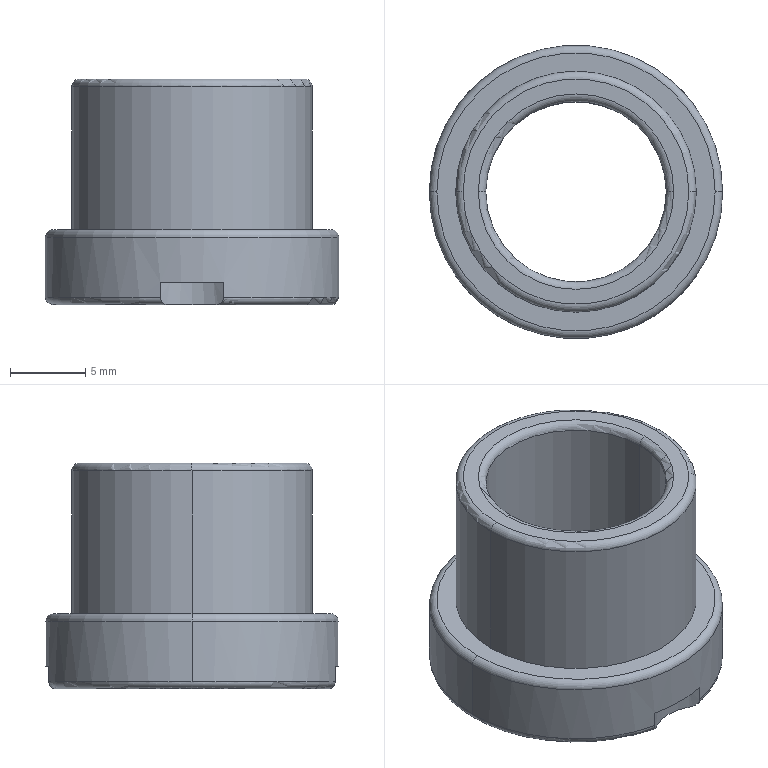Part | SolidWorks | features BaseBody 1 | 1 solid | 24 faces | box 19.5 x 19.5 x 15 mm | volume 1786 mm3 | torus 11 | cylinder 8 | plane 5 | commonest cylinder face diameters 6.5 x2 12 x2 16 x2 19.5 x2
STEP:
#1=CARTESIAN_POINT('',(-8.,0.,14.5));
#2=VERTEX_POINT('',#1);
#3=CARTESIAN_POINT('',(8.,0.,14.5));
#4=VERTEX_POINT('',#3);
#5=CARTESIAN_POINT('',(0.,0.,14.5));
#6=DIRECTION('',(0.,0.,-1.));
#7=DIRECTION('',(1.,0.,0.));
#8=AXIS2_PLACEMENT_3D('',#5,#6,#7);
#9=CIRCLE('',#8,8.);
#10=EDGE_CURVE('',#2,#4,#9,.T.);
#11=ORIENTED_EDGE('',*,*,#10,.F.);
#12=CARTESIAN_POINT('',(-7.5,0.,15.));
#13=VERTEX_POINT('',#12);
#14=CARTESIAN_POINT('',(-7.5,0.,14.5));
#15=DIRECTION('',(0.,1.,0.));
#16=DIRECTION('',(-1.,0.,0.));
#17=AXIS2_PLACEMENT_3D('',#14,#15,#16);
#18=CIRCLE('',#17,0.5);
#19=EDGE_CURVE('',#2,#13,#18,.T.);
#20=ORIENTED_EDGE('',*,*,#19,.T.);
#21=CARTESIAN_POINT('',(7.5,0.,15.));
#22=VERTEX_POINT('',#21);
#23=CARTESIAN_POINT('',(0.,0.,15.));
#24=DIRECTION('',(0.,0.,1.));
#25=DIRECTION('',(1.,0.,0.));
#26=AXIS2_PLACEMENT_3D('',#23,#24,#25);
#27=CIRCLE('',#26,7.5);
#28=EDGE_CURVE('',#22,#13,#27,.T.);
#29=ORIENTED_EDGE('',*,*,#28,.F.);
#30=CARTESIAN_POINT('',(7.5,0.,14.5));
#31=DIRECTION('',(0.,-1.,0.));
#32=DIRECTION('',(0.,0.,-1.));
#33=AXIS2_PLACEMENT_3D('',#30,#31,#32);
#34=CIRCLE('',#33,0.5);
#35=EDGE_CURVE('',#4,#22,#34,.T.);
#36=ORIENTED_EDGE('',*,*,#35,.F.);
#37=EDGE_LOOP('',(#11,#20,#29,#36));
#38=FACE_OUTER_BOUND('',#37,.T.);
#39=CARTESIAN_POINT('',(0.,0.,14.5));
#40=DIRECTION('',(0.,0.,1.));
#41=DIRECTION('',(1.,0.,0.));
#42=AXIS2_PLACEMENT_3D('',#39,#40,#41);
#43=TOROIDAL_SURFACE('',#42,7.5,0.5);
#44=ADVANCED_FACE('',(#38),#43,.T.);
#45=CARTESIAN_POINT('',(9.25,0.,5.));
#46=VERTEX_POINT('',#45);
#47=CARTESIAN_POINT('',(-9.25,0.,5.));
#48=VERTEX_POINT('',#47);
#49=CARTESIAN_POINT('',(0.,0.,5.));
#50=DIRECTION('',(0.,0.,1.));
#51=DIRECTION('',(-1.,0.,0.));
#52=AXIS2_PLACEMENT_3D('',#49,#50,#51);
#53=CIRCLE('',#52,9.25);
#54=EDGE_CURVE('',#46,#48,#53,.T.);
#55=ORIENTED_EDGE('',*,*,#54,.F.);
#56=CARTESIAN_POINT('',(9.75,0.,4.5));
#57=VERTEX_POINT('',#56);
#58=CARTESIAN_POINT('',(9.25,0.,4.5));
#59=DIRECTION('',(0.,1.,0.));
#60=DIRECTION('',(-1.,0.,0.));
#61=AXIS2_PLACEMENT_3D('',#58,#59,#60);
#62=CIRCLE('',#61,0.5);
#63=EDGE_CURVE('',#46,#57,#62,.T.);
#64=ORIENTED_EDGE('',*,*,#63,.T.);
#65=CARTESIAN_POINT('',(-9.75,0.,4.5));
#66=VERTEX_POINT('',#65);
#67=CARTESIAN_POINT('',(0.,0.,4.5));
#68=DIRECTION('',(0.,0.,-1.));
#69=DIRECTION('',(-1.,0.,0.));
#70=AXIS2_PLACEMENT_3D('',#67,#68,#69);
#71=CIRCLE('',#70,9.75);
#72=EDGE_CURVE('',#66,#57,#71,.T.);
#73=ORIENTED_EDGE('',*,*,#72,.F.);
#74=CARTESIAN_POINT('',(-9.25,0.,4.5));
#75=DIRECTION('',(0.,-1.,0.));
#76=DIRECTION('',(0.,0.,-1.));
#77=AXIS2_PLACEMENT_3D('',#74,#75,#76);
#78=CIRCLE('',#77,0.5);
#79=EDGE_CURVE('',#48,#66,#78,.T.);
#80=ORIENTED_EDGE('',*,*,#79,.F.);
#81=EDGE_LOOP('',(#55,#64,#73,#80));
#82=FACE_OUTER_BOUND('',#81,.T.);
#83=CARTESIAN_POINT('',(0.,0.,4.5));
#84=DIRECTION('',(0.,0.,-1.));
#85=DIRECTION('',(-1.,0.,0.));
#86=AXIS2_PLACEMENT_3D('',#83,#84,#85);
#87=TOROIDAL_SURFACE('',#86,9.25,0.5);
#88=ADVANCED_FACE('',(#82),#87,.T.);
#89=CARTESIAN_POINT('',(9.25,0.,0.));
#90=VERTEX_POINT('',#89);
#91=CARTESIAN_POINT('',(1.516,-9.125,0.));
#92=VERTEX_POINT('',#91);
#93=CARTESIAN_POINT('',(0.,0.,0.));
#94=DIRECTION('',(0.,0.,-1.));
#95=DIRECTION('',(1.,0.,0.));
#96=AXIS2_PLACEMENT_3D('',#93,#94,#95);
#97=CIRCLE('',#96,9.25);
#98=EDGE_CURVE('',#90,#92,#97,.T.);
#99=ORIENTED_EDGE('',*,*,#98,.F.);
#100=CARTESIAN_POINT('',(9.75,0.,0.5));
#101=VERTEX_POINT('',#100);
#102=CARTESIAN_POINT('',(9.25,0.,0.5));
#103=DIRECTION('',(0.,-1.,0.));
#104=DIRECTION('',(0.,0.,-1.));
#105=AXIS2_PLACEMENT_3D('',#102,#103,#104);
#106=CIRCLE('',#105,0.5);
#107=EDGE_CURVE('',#90,#101,#106,.T.);
#108=ORIENTED_EDGE('',*,*,#107,.T.);
#109=CARTESIAN_POINT('',(2.101,-9.521,0.5));
#110=VERTEX_POINT('',#109);
#111=CARTESIAN_POINT('',(0.,0.,0.5));
#112=DIRECTION('',(0.,0.,1.));
#113=DIRECTION('',(1.,0.,0.));
#114=AXIS2_PLACEMENT_3D('',#111,#112,#113);
#115=CIRCLE('',#114,9.75);
#116=EDGE_CURVE('',#110,#101,#115,.T.);
#117=ORIENTED_EDGE('',*,*,#116,.F.);
#118=CARTESIAN_POINT('',(1.516,-9.125,0.));
#119=CARTESIAN_POINT('',(1.587,-9.163,0.));
#120=CARTESIAN_POINT('',(1.656,-9.202,0.006968));
#121=CARTESIAN_POINT('',(1.788,-9.285,0.04068));
#122=CARTESIAN_POINT('',(1.852,-9.328,0.06811));
#123=CARTESIAN_POINT('',(1.964,-9.41,0.1494));
#124=CARTESIAN_POINT('',(2.013,-9.448,0.2038));
#125=CARTESIAN_POINT('',(2.082,-9.504,0.3397));
#126=CARTESIAN_POINT('',(2.101,-9.521,0.4184));
#127=CARTESIAN_POINT('',(2.101,-9.521,0.5));
#128=B_SPLINE_CURVE_WITH_KNOTS('',3,(#118,#119,#120,#121,#122,#123,#124,#125,#126,#127),.UNSPECIFIED.,.F.,.F.,(4,2,2,2,4),(0.,0.0002386,0.0004771,0.0007157,0.0009543),.UNSPECIFIED.);
#129=EDGE_CURVE('',#92,#110,#128,.T.);
#130=ORIENTED_EDGE('',*,*,#129,.F.);
#131=EDGE_LOOP('',(#99,#108,#117,#130));
#132=FACE_OUTER_BOUND('',#131,.T.);
#133=CARTESIAN_POINT('',(0.,0.,0.5));
#134=DIRECTION('',(0.,0.,1.));
#135=DIRECTION('',(1.,0.,0.));
#136=AXIS2_PLACEMENT_3D('',#133,#134,#135);
#137=TOROIDAL_SURFACE('',#136,9.25,0.5);
#138=ADVANCED_FACE('',(#132),#137,.T.);
#139=CARTESIAN_POINT('',(-6.5,0.,15.));
#140=VERTEX_POINT('',#139);
#141=CARTESIAN_POINT('',(6.5,0.,15.));
#142=VERTEX_POINT('',#141);
#143=CARTESIAN_POINT('',(0.,0.,15.));
#144=DIRECTION('',(0.,0.,-1.));
#145=DIRECTION('',(1.,0.,0.));
#146=AXIS2_PLACEMENT_3D('',#143,#144,#145);
#147=CIRCLE('',#146,6.5);
#148=EDGE_CURVE('',#140,#142,#147,.T.);
#149=ORIENTED_EDGE('',*,*,#148,.F.);
#150=CARTESIAN_POINT('',(-6.,0.,14.5));
#151=VERTEX_POINT('',#150);
#152=CARTESIAN_POINT('',(-6.5,0.,14.5));
#153=DIRECTION('',(0.,1.,0.));
#154=DIRECTION('',(-1.,0.,0.));
#155=AXIS2_PLACEMENT_3D('',#152,#153,#154);
#156=CIRCLE('',#155,0.5);
#157=EDGE_CURVE('',#140,#151,#156,.T.);
#158=ORIENTED_EDGE('',*,*,#157,.T.);
#159=CARTESIAN_POINT('',(6.,0.,14.5));
#160=VERTEX_POINT('',#159);
#161=CARTESIAN_POINT('',(0.,0.,14.5));
#162=DIRECTION('',(0.,0.,1.));
#163=DIRECTION('',(1.,0.,0.));
#164=AXIS2_PLACEMENT_3D('',#161,#162,#163);
#165=CIRCLE('',#164,6.);
#166=EDGE_CURVE('',#160,#151,#165,.T.);
#167=ORIENTED_EDGE('',*,*,#166,.F.);
#168=CARTESIAN_POINT('',(6.5,0.,14.5));
#169=DIRECTION('',(0.,-1.,0.));
#170=DIRECTION('',(0.,0.,-1.));
#171=AXIS2_PLACEMENT_3D('',#168,#169,#170);
#172=CIRCLE('',#171,0.5);
#173=EDGE_CURVE('',#142,#160,#172,.T.);
#174=ORIENTED_EDGE('',*,*,#173,.F.);
#175=EDGE_LOOP('',(#149,#158,#167,#174));
#176=FACE_OUTER_BOUND('',#175,.T.);
#177=CARTESIAN_POINT('',(0.,0.,14.5));
#178=DIRECTION('',(0.,0.,1.));
#179=DIRECTION('',(1.,0.,0.));
#180=AXIS2_PLACEMENT_3D('',#177,#178,#179);
#181=TOROIDAL_SURFACE('',#180,6.5,0.5);
#182=ADVANCED_FACE('',(#176),#181,.T.);
#183=CARTESIAN_POINT('',(-6.,0.,0.5));
#184=VERTEX_POINT('',#183);
#185=CARTESIAN_POINT('',(6.,0.,0.5));
#186=VERTEX_POINT('',#185);
#187=CARTESIAN_POINT('',(0.,0.,0.5));
#188=DIRECTION('',(0.,0.,-1.));
#189=DIRECTION('',(1.,0.,0.));
#190=AXIS2_PLACEMENT_3D('',#187,#188,#189);
#191=CIRCLE('',#190,6.);
#192=EDGE_CURVE('',#184,#186,#191,.T.);
#193=ORIENTED_EDGE('',*,*,#192,.F.);
#194=CARTESIAN_POINT('',(-6.5,0.,0.));
#195=VERTEX_POINT('',#194);
#196=CARTESIAN_POINT('',(-6.5,0.,0.5));
#197=DIRECTION('',(0.,1.,0.));
#198=DIRECTION('',(-1.,0.,0.));
#199=AXIS2_PLACEMENT_3D('',#196,#197,#198);
#200=CIRCLE('',#199,0.5);
#201=EDGE_CURVE('',#184,#195,#200,.T.);
#202=ORIENTED_EDGE('',*,*,#201,.T.);
#203=CARTESIAN_POINT('',(6.5,0.,0.));
#204=VERTEX_POINT('',#203);
#205=CARTESIAN_POINT('',(0.,0.,0.));
#206=DIRECTION('',(0.,0.,1.));
#207=DIRECTION('',(1.,0.,0.));
#208=AXIS2_PLACEMENT_3D('',#205,#206,#207);
#209=CIRCLE('',#208,6.5);
#210=EDGE_CURVE('',#204,#195,#209,.T.);
#211=ORIENTED_EDGE('',*,*,#210,.F.);
#212=CARTESIAN_POINT('',(6.5,0.,0.5));
#213=DIRECTION('',(0.,-1.,0.));
#214=DIRECTION('',(0.,0.,-1.));
#215=AXIS2_PLACEMENT_3D('',#212,#213,#214);
#216=CIRCLE('',#215,0.5);
#217=EDGE_CURVE('',#186,#204,#216,.T.);
#218=ORIENTED_EDGE('',*,*,#217,.F.);
#219=EDGE_LOOP('',(#193,#202,#211,#218));
#220=FACE_OUTER_BOUND('',#219,.T.);
#221=CARTESIAN_POINT('',(0.,0.,0.5));
#222=DIRECTION('',(0.,0.,1.));
#223=DIRECTION('',(1.,0.,0.));
#224=AXIS2_PLACEMENT_3D('',#221,#222,#223);
#225=TOROIDAL_SURFACE('',#224,6.5,0.5);
#226=ADVANCED_FACE('',(#220),#225,.T.);
#227=ORIENTED_EDGE('',*,*,#72,.T.);
#228=CARTESIAN_POINT('',(9.75,0.,5.));
#229=DIRECTION('',(0.,0.,-1.));
#230=VECTOR('',#229,1000.);
#231=LINE('',#228,#230);
#232=EDGE_CURVE('',#57,#101,#231,.T.);
#233=ORIENTED_EDGE('',*,*,#232,.T.);
#234=CARTESIAN_POINT('',(2.101,9.521,0.5));
#235=VERTEX_POINT('',#234);
#236=CARTESIAN_POINT('',(0.,0.,0.5));
#237=DIRECTION('',(0.,0.,1.));
#238=DIRECTION('',(1.,0.,0.));
#239=AXIS2_PLACEMENT_3D('',#236,#237,#238);
#240=CIRCLE('',#239,9.75);
#241=EDGE_CURVE('',#101,#235,#240,.T.);
#242=ORIENTED_EDGE('',*,*,#241,.T.);
#243=CARTESIAN_POINT('',(2.101,9.521,1.5));
#244=VERTEX_POINT('',#243);
#245=CARTESIAN_POINT('',(2.101,9.521,0.75));
#246=DIRECTION('',(0.,0.,-1.));
#247=VECTOR('',#246,1000.);
#248=LINE('',#245,#247);
#249=EDGE_CURVE('',#244,#235,#248,.T.);
#250=ORIENTED_EDGE('',*,*,#249,.F.);
#251=CARTESIAN_POINT('',(-2.101,9.521,1.5));
#252=VERTEX_POINT('',#251);
#253=CARTESIAN_POINT('',(0.,0.,1.5));
#254=DIRECTION('',(0.,0.,1.));
#255=DIRECTION('',(-1.,0.,0.));
#256=AXIS2_PLACEMENT_3D('',#253,#254,#255);
#257=CIRCLE('',#256,9.75);
#258=EDGE_CURVE('',#244,#252,#257,.T.);
#259=ORIENTED_EDGE('',*,*,#258,.T.);
#260=CARTESIAN_POINT('',(-2.101,9.521,0.5));
#261=VERTEX_POINT('',#260);
#262=CARTESIAN_POINT('',(-2.101,9.521,0.75));
#263=DIRECTION('',(0.,0.,1.));
#264=VECTOR('',#263,1000.);
#265=LINE('',#262,#264);
#266=EDGE_CURVE('',#261,#252,#265,.T.);
#267=ORIENTED_EDGE('',*,*,#266,.F.);
#268=CARTESIAN_POINT('',(-9.75,0.,0.5));
#269=VERTEX_POINT('',#268);
#270=CARTESIAN_POINT('',(0.,0.,0.5));
#271=DIRECTION('',(0.,0.,1.));
#272=DIRECTION('',(1.,0.,0.));
#273=AXIS2_PLACEMENT_3D('',#270,#271,#272);
#274=CIRCLE('',#273,9.75);
#275=EDGE_CURVE('',#261,#269,#274,.T.);
#276=ORIENTED_EDGE('',*,*,#275,.T.);
#277=CARTESIAN_POINT('',(-9.75,0.,5.));
#278=DIRECTION('',(0.,0.,-1.));
#279=VECTOR('',#278,1000.);
#280=LINE('',#277,#279);
#281=EDGE_CURVE('',#66,#269,#280,.T.);
#282=ORIENTED_EDGE('',*,*,#281,.F.);
#283=EDGE_LOOP('',(#227,#233,#242,#250,#259,#267,#276,#282));
#284=FACE_OUTER_BOUND('',#283,.T.);
#285=CARTESIAN_POINT('',(0.,0.,5.));
#286=DIRECTION('',(0.,0.,-1.));
#287=DIRECTION('',(-1.,0.,0.));
#288=AXIS2_PLACEMENT_3D('',#285,#286,#287);
#289=CYLINDRICAL_SURFACE('',#288,9.75);
#290=ADVANCED_FACE('',(#284),#289,.T.);
#291=CARTESIAN_POINT('',(0.,0.,14.5));
#292=DIRECTION('',(0.,0.,1.));
#293=DIRECTION('',(1.,0.,0.));
#294=AXIS2_PLACEMENT_3D('',#291,#292,#293);
#295=CIRCLE('',#294,6.);
#296=EDGE_CURVE('',#151,#160,#295,.T.);
#297=ORIENTED_EDGE('',*,*,#296,.T.);
#298=CARTESIAN_POINT('',(6.,0.,15.));
#299=DIRECTION('',(0.,0.,-1.));
#300=VECTOR('',#299,1000.);
#301=LINE('',#298,#300);
#302=EDGE_CURVE('',#160,#186,#301,.T.);
#303=ORIENTED_EDGE('',*,*,#302,.T.);
#304=CARTESIAN_POINT('',(0.,0.,0.5));
#305=DIRECTION('',(0.,0.,-1.));
#306=DIRECTION('',(1.,0.,0.));
#307=AXIS2_PLACEMENT_3D('',#304,#305,#306);
#308=CIRCLE('',#307,6.);
#309=EDGE_CURVE('',#186,#184,#308,.T.);
#310=ORIENTED_EDGE('',*,*,#309,.T.);
#311=CARTESIAN_POINT('',(-6.,0.,15.));
#312=DIRECTION('',(0.,0.,-1.));
#313=VECTOR('',#312,1000.);
#314=LINE('',#311,#313);
#315=EDGE_CURVE('',#151,#184,#314,.T.);
#316=ORIENTED_EDGE('',*,*,#315,.F.);
#317=EDGE_LOOP('',(#297,#303,#310,#316));
#318=FACE_OUTER_BOUND('',#317,.T.);
#319=CARTESIAN_POINT('',(0.,0.,15.));
#320=DIRECTION('',(0.,0.,-1.));
#321=DIRECTION('',(-1.,0.,0.));
#322=AXIS2_PLACEMENT_3D('',#319,#320,#321);
#323=CYLINDRICAL_SURFACE('',#322,6.);
#324=ADVANCED_FACE('',(#318),#323,.F.);
#325=ORIENTED_EDGE('',*,*,#10,.T.);
#326=CARTESIAN_POINT('',(8.,0.,5.));
#327=VERTEX_POINT('',#326);
#328=CARTESIAN_POINT('',(8.,0.,15.));
#329=DIRECTION('',(0.,0.,-1.));
#330=VECTOR('',#329,1000.);
#331=LINE('',#328,#330);
#332=EDGE_CURVE('',#4,#327,#331,.T.);
#333=ORIENTED_EDGE('',*,*,#332,.T.);
#334=CARTESIAN_POINT('',(-8.,0.,5.));
#335=VERTEX_POINT('',#334);
#336=CARTESIAN_POINT('',(0.,0.,5.));
#337=DIRECTION('',(0.,0.,-1.));
#338=DIRECTION('',(-1.,0.,0.));
#339=AXIS2_PLACEMENT_3D('',#336,#337,#338);
#340=CIRCLE('',#339,8.);
#341=EDGE_CURVE('',#335,#327,#340,.T.);
#342=ORIENTED_EDGE('',*,*,#341,.F.);
#343=CARTESIAN_POINT('',(-8.,0.,15.));
#344=DIRECTION('',(0.,0.,-1.));
#345=VECTOR('',#344,1000.);
#346=LINE('',#343,#345);
#347=EDGE_CURVE('',#2,#335,#346,.T.);
#348=ORIENTED_EDGE('',*,*,#347,.F.);
#349=EDGE_LOOP('',(#325,#333,#342,#348));
#350=FACE_OUTER_BOUND('',#349,.T.);
#351=CARTESIAN_POINT('',(0.,0.,15.));
#352=DIRECTION('',(0.,0.,-1.));
#353=DIRECTION('',(-1.,0.,0.));
#354=AXIS2_PLACEMENT_3D('',#351,#352,#353);
#355=CYLINDRICAL_SURFACE('',#354,8.);
#356=ADVANCED_FACE('',(#350),#355,.T.);
#357=CARTESIAN_POINT('',(0.,12.,1.5));
#358=DIRECTION('',(0.,0.,-1.));
#359=DIRECTION('',(-1.,0.,0.));
#360=AXIS2_PLACEMENT_3D('',#357,#358,#359);
#361=CIRCLE('',#360,3.25);
#362=EDGE_CURVE('',#244,#252,#361,.T.);
#363=ORIENTED_EDGE('',*,*,#362,.T.);
#364=ORIENTED_EDGE('',*,*,#258,.F.);
#365=EDGE_LOOP('',(#363,#364));
#366=FACE_OUTER_BOUND('',#365,.T.);
#367=CARTESIAN_POINT('',(0.,12.,1.5));
#368=DIRECTION('',(0.,0.,-1.));
#369=DIRECTION('',(0.,-1.,0.));
#370=AXIS2_PLACEMENT_3D('',#367,#368,#369);
#371=PLANE('',#370);
#372=ADVANCED_FACE('',(#366),#371,.T.);
#373=ORIENTED_EDGE('',*,*,#266,.T.);
#374=ORIENTED_EDGE('',*,*,#362,.F.);
#375=ORIENTED_EDGE('',*,*,#249,.T.);
#376=CARTESIAN_POINT('',(1.516,9.125,0.));
#377=VERTEX_POINT('',#376);
#378=CARTESIAN_POINT('',(2.101,9.521,0.5));
#379=CARTESIAN_POINT('',(2.101,9.521,0.4186));
#380=CARTESIAN_POINT('',(2.082,9.504,0.3394));
#381=CARTESIAN_POINT('',(2.014,9.448,0.2048));
#382=CARTESIAN_POINT('',(1.964,9.41,0.1496));
#383=CARTESIAN_POINT('',(1.852,9.329,0.06829));
#384=CARTESIAN_POINT('',(1.789,9.285,0.04095));
#385=CARTESIAN_POINT('',(1.656,9.202,0.006954));
#386=CARTESIAN_POINT('',(1.587,9.163,0.));
#387=CARTESIAN_POINT('',(1.516,9.125,0.));
#388=B_SPLINE_CURVE_WITH_KNOTS('',3,(#378,#379,#380,#381,#382,#383,#384,#385,#386,#387),.UNSPECIFIED.,.F.,.F.,(4,2,2,2,4),(0.,0.0002405,0.000481,0.0007214,0.0009619),.UNSPECIFIED.);
#389=EDGE_CURVE('',#235,#377,#388,.T.);
#390=ORIENTED_EDGE('',*,*,#389,.T.);
#391=CARTESIAN_POINT('',(-1.516,9.125,0.));
#392=VERTEX_POINT('',#391);
#393=CARTESIAN_POINT('',(0.,12.,0.));
#394=DIRECTION('',(0.,0.,-1.));
#395=DIRECTION('',(-1.,0.,0.));
#396=AXIS2_PLACEMENT_3D('',#393,#394,#395);
#397=CIRCLE('',#396,3.25);
#398=EDGE_CURVE('',#377,#392,#397,.T.);
#399=ORIENTED_EDGE('',*,*,#398,.T.);
#400=CARTESIAN_POINT('',(-1.516,9.125,0.));
#401=CARTESIAN_POINT('',(-1.587,9.163,0.));
#402=CARTESIAN_POINT('',(-1.656,9.202,0.006968));
#403=CARTESIAN_POINT('',(-1.788,9.285,0.04068));
#404=CARTESIAN_POINT('',(-1.852,9.328,0.06811));
#405=CARTESIAN_POINT('',(-1.964,9.41,0.1494));
#406=CARTESIAN_POINT('',(-2.013,9.448,0.2038));
#407=CARTESIAN_POINT('',(-2.082,9.504,0.3397));
#408=CARTESIAN_POINT('',(-2.101,9.521,0.4184));
#409=CARTESIAN_POINT('',(-2.101,9.521,0.5));
#410=B_SPLINE_CURVE_WITH_KNOTS('',3,(#400,#401,#402,#403,#404,#405,#406,#407,#408,#409),.UNSPECIFIED.,.F.,.F.,(4,2,2,2,4),(0.,0.0002386,0.0004771,0.0007157,0.0009543),.UNSPECIFIED.);
#411=EDGE_CURVE('',#392,#261,#410,.T.);
#412=ORIENTED_EDGE('',*,*,#411,.T.);
#413=EDGE_LOOP('',(#373,#374,#375,#390,#399,#412));
#414=FACE_OUTER_BOUND('',#413,.T.);
#415=CARTESIAN_POINT('',(0.,12.,1.5));
#416=DIRECTION('',(0.,0.,-1.));
#417=DIRECTION('',(-1.,0.,0.));
#418=AXIS2_PLACEMENT_3D('',#415,#416,#417);
#419=CYLINDRICAL_SURFACE('',#418,3.25);
#420=ADVANCED_FACE('',(#414),#419,.F.);
#421=CARTESIAN_POINT('',(-2.101,-9.521,1.5));
#422=VERTEX_POINT('',#421);
#423=CARTESIAN_POINT('',(2.101,-9.521,1.5));
#424=VERTEX_POINT('',#423);
#425=CARTESIAN_POINT('',(0.,-12.,1.5));
#426=DIRECTION('',(0.,0.,-1.));
#427=DIRECTION('',(-1.,0.,0.));
#428=AXIS2_PLACEMENT_3D('',#425,#426,#427);
#429=CIRCLE('',#428,3.25);
#430=EDGE_CURVE('',#422,#424,#429,.T.);
#431=ORIENTED_EDGE('',*,*,#430,.T.);
#432=CARTESIAN_POINT('',(0.,0.,1.5));
#433=DIRECTION('',(0.,0.,1.));
#434=DIRECTION('',(-1.,0.,0.));
#435=AXIS2_PLACEMENT_3D('',#432,#433,#434);
#436=CIRCLE('',#435,9.75);
#437=EDGE_CURVE('',#422,#424,#436,.T.);
#438=ORIENTED_EDGE('',*,*,#437,.F.);
#439=EDGE_LOOP('',(#431,#438));
#440=FACE_OUTER_BOUND('',#439,.T.);
#441=CARTESIAN_POINT('',(0.,-12.,1.5));
#442=DIRECTION('',(0.,0.,-1.));
#443=DIRECTION('',(0.,-1.,0.));
#444=AXIS2_PLACEMENT_3D('',#441,#442,#443);
#445=PLANE('',#444);
#446=ADVANCED_FACE('',(#440),#445,.T.);
#447=CARTESIAN_POINT('',(2.101,-9.521,0.75));
#448=DIRECTION('',(0.,0.,1.));
#449=VECTOR('',#448,1000.);
#450=LINE('',#447,#449);
#451=EDGE_CURVE('',#110,#424,#450,.T.);
#452=ORIENTED_EDGE('',*,*,#451,.T.);
#453=ORIENTED_EDGE('',*,*,#430,.F.);
#454=CARTESIAN_POINT('',(-2.101,-9.521,0.5));
#455=VERTEX_POINT('',#454);
#456=CARTESIAN_POINT('',(-2.101,-9.521,0.75));
#457=DIRECTION('',(0.,0.,-1.));
#458=VECTOR('',#457,1000.);
#459=LINE('',#456,#458);
#460=EDGE_CURVE('',#422,#455,#459,.T.);
#461=ORIENTED_EDGE('',*,*,#460,.T.);
#462=CARTESIAN_POINT('',(-1.516,-9.125,0.));
#463=VERTEX_POINT('',#462);
#464=CARTESIAN_POINT('',(-2.101,-9.521,0.5));
#465=CARTESIAN_POINT('',(-2.101,-9.521,0.4186));
#466=CARTESIAN_POINT('',(-2.082,-9.504,0.3394));
#467=CARTESIAN_POINT('',(-2.014,-9.448,0.2048));
#468=CARTESIAN_POINT('',(-1.964,-9.41,0.1496));
#469=CARTESIAN_POINT('',(-1.852,-9.329,0.06829));
#470=CARTESIAN_POINT('',(-1.789,-9.285,0.04095));
#471=CARTESIAN_POINT('',(-1.656,-9.202,0.006954));
#472=CARTESIAN_POINT('',(-1.587,-9.163,0.));
#473=CARTESIAN_POINT('',(-1.516,-9.125,0.));
#474=B_SPLINE_CURVE_WITH_KNOTS('',3,(#464,#465,#466,#467,#468,#469,#470,#471,#472,#473),.UNSPECIFIED.,.F.,.F.,(4,2,2,2,4),(0.,0.0002405,0.000481,0.0007214,0.0009619),.UNSPECIFIED.);
#475=EDGE_CURVE('',#455,#463,#474,.T.);
#476=ORIENTED_EDGE('',*,*,#475,.T.);
#477=CARTESIAN_POINT('',(0.,-12.,0.));
#478=DIRECTION('',(0.,0.,-1.));
#479=DIRECTION('',(-1.,0.,0.));
#480=AXIS2_PLACEMENT_3D('',#477,#478,#479);
#481=CIRCLE('',#480,3.25);
#482=EDGE_CURVE('',#463,#92,#481,.T.);
#483=ORIENTED_EDGE('',*,*,#482,.T.);
#484=ORIENTED_EDGE('',*,*,#129,.T.);
#485=EDGE_LOOP('',(#452,#453,#461,#476,#483,#484));
#486=FACE_OUTER_BOUND('',#485,.T.);
#487=CARTESIAN_POINT('',(0.,-12.,1.5));
#488=DIRECTION('',(0.,0.,-1.));
#489=DIRECTION('',(-1.,0.,0.));
#490=AXIS2_PLACEMENT_3D('',#487,#488,#489);
#491=CYLINDRICAL_SURFACE('',#490,3.25);
#492=ADVANCED_FACE('',(#486),#491,.F.);
#493=ORIENTED_EDGE('',*,*,#341,.T.);
#494=CARTESIAN_POINT('',(0.,0.,5.));
#495=DIRECTION('',(0.,0.,-1.));
#496=DIRECTION('',(-1.,0.,0.));
#497=AXIS2_PLACEMENT_3D('',#494,#495,#496);
#498=CIRCLE('',#497,8.);
#499=EDGE_CURVE('',#327,#335,#498,.T.);
#500=ORIENTED_EDGE('',*,*,#499,.T.);
#501=EDGE_LOOP('',(#493,#500));
#502=FACE_BOUND('',#501,.T.);
#503=CARTESIAN_POINT('',(0.,0.,5.));
#504=DIRECTION('',(0.,0.,1.));
#505=DIRECTION('',(-1.,0.,0.));
#506=AXIS2_PLACEMENT_3D('',#503,#504,#505);
#507=CIRCLE('',#506,9.25);
#508=EDGE_CURVE('',#48,#46,#507,.T.);
#509=ORIENTED_EDGE('',*,*,#508,.T.);
#510=ORIENTED_EDGE('',*,*,#54,.T.);
#511=EDGE_LOOP('',(#509,#510));
#512=FACE_OUTER_BOUND('',#511,.T.);
#513=CARTESIAN_POINT('',(0.,0.,5.));
#514=DIRECTION('',(0.,0.,-1.));
#515=DIRECTION('',(0.,-1.,0.));
#516=AXIS2_PLACEMENT_3D('',#513,#514,#515);
#517=PLANE('',#516);
#518=ADVANCED_FACE('',(#502,#512),#517,.F.);
#519=ORIENTED_EDGE('',*,*,#210,.T.);
#520=CARTESIAN_POINT('',(0.,0.,0.));
#521=DIRECTION('',(0.,0.,1.));
#522=DIRECTION('',(1.,0.,0.));
#523=AXIS2_PLACEMENT_3D('',#520,#521,#522);
#524=CIRCLE('',#523,6.5);
#525=EDGE_CURVE('',#195,#204,#524,.T.);
#526=ORIENTED_EDGE('',*,*,#525,.T.);
#527=EDGE_LOOP('',(#519,#526));
#528=FACE_BOUND('',#527,.T.);
#529=CARTESIAN_POINT('',(0.,0.,0.));
#530=DIRECTION('',(0.,0.,-1.));
#531=DIRECTION('',(1.,0.,0.));
#532=AXIS2_PLACEMENT_3D('',#529,#530,#531);
#533=CIRCLE('',#532,9.25);
#534=EDGE_CURVE('',#463,#392,#533,.T.);
#535=ORIENTED_EDGE('',*,*,#534,.T.);
#536=ORIENTED_EDGE('',*,*,#398,.F.);
#537=CARTESIAN_POINT('',(0.,0.,0.));
#538=DIRECTION('',(0.,0.,-1.));
#539=DIRECTION('',(1.,0.,0.));
#540=AXIS2_PLACEMENT_3D('',#537,#538,#539);
#541=CIRCLE('',#540,9.25);
#542=EDGE_CURVE('',#377,#90,#541,.T.);
#543=ORIENTED_EDGE('',*,*,#542,.T.);
#544=ORIENTED_EDGE('',*,*,#98,.T.);
#545=ORIENTED_EDGE('',*,*,#482,.F.);
#546=EDGE_LOOP('',(#535,#536,#543,#544,#545));
#547=FACE_OUTER_BOUND('',#546,.T.);
#548=CARTESIAN_POINT('',(0.,0.,0.));
#549=DIRECTION('',(0.,0.,1.));
#550=DIRECTION('',(1.,0.,0.));
#551=AXIS2_PLACEMENT_3D('',#548,#549,#550);
#552=PLANE('',#551);
#553=ADVANCED_FACE('',(#528,#547),#552,.F.);
#554=CARTESIAN_POINT('',(0.,0.,15.));
#555=DIRECTION('',(0.,0.,-1.));
#556=DIRECTION('',(1.,0.,0.));
#557=AXIS2_PLACEMENT_3D('',#554,#555,#556);
#558=CIRCLE('',#557,6.5);
#559=EDGE_CURVE('',#142,#140,#558,.T.);
#560=ORIENTED_EDGE('',*,*,#559,.T.);
#561=ORIENTED_EDGE('',*,*,#148,.T.);
#562=EDGE_LOOP('',(#560,#561));
#563=FACE_BOUND('',#562,.T.);
#564=ORIENTED_EDGE('',*,*,#28,.T.);
#565=CARTESIAN_POINT('',(0.,0.,15.));
#566=DIRECTION('',(0.,0.,1.));
#567=DIRECTION('',(1.,0.,0.));
#568=AXIS2_PLACEMENT_3D('',#565,#566,#567);
#569=CIRCLE('',#568,7.5);
#570=EDGE_CURVE('',#13,#22,#569,.T.);
#571=ORIENTED_EDGE('',*,*,#570,.T.);
#572=EDGE_LOOP('',(#564,#571));
#573=FACE_OUTER_BOUND('',#572,.T.);
#574=CARTESIAN_POINT('',(0.,0.,15.));
#575=DIRECTION('',(0.,0.,1.));
#576=DIRECTION('',(1.,0.,0.));
#577=AXIS2_PLACEMENT_3D('',#574,#575,#576);
#578=PLANE('',#577);
#579=ADVANCED_FACE('',(#563,#573),#578,.T.);
#580=ORIENTED_EDGE('',*,*,#411,.F.);
#581=ORIENTED_EDGE('',*,*,#534,.F.);
#582=ORIENTED_EDGE('',*,*,#475,.F.);
#583=CARTESIAN_POINT('',(0.,0.,0.5));
#584=DIRECTION('',(0.,0.,1.));
#585=DIRECTION('',(1.,0.,0.));
#586=AXIS2_PLACEMENT_3D('',#583,#584,#585);
#587=CIRCLE('',#586,9.75);
#588=EDGE_CURVE('',#269,#455,#587,.T.);
#589=ORIENTED_EDGE('',*,*,#588,.F.);
#590=ORIENTED_EDGE('',*,*,#275,.F.);
#591=EDGE_LOOP('',(#580,#581,#582,#589,#590));
#592=FACE_OUTER_BOUND('',#591,.T.);
#593=CARTESIAN_POINT('',(0.,0.,0.5));
#594=DIRECTION('',(0.,0.,1.));
#595=DIRECTION('',(1.,0.,0.));
#596=AXIS2_PLACEMENT_3D('',#593,#594,#595);
#597=TOROIDAL_SURFACE('',#596,9.25,0.5);
#598=ADVANCED_FACE('',(#592),#597,.T.);
#599=ORIENTED_EDGE('',*,*,#332,.F.);
#600=CARTESIAN_POINT('',(0.,0.,14.5));
#601=DIRECTION('',(0.,0.,-1.));
#602=DIRECTION('',(1.,0.,0.));
#603=AXIS2_PLACEMENT_3D('',#600,#601,#602);
#604=CIRCLE('',#603,8.);
#605=EDGE_CURVE('',#4,#2,#604,.T.);
#606=ORIENTED_EDGE('',*,*,#605,.T.);
#607=ORIENTED_EDGE('',*,*,#347,.T.);
#608=ORIENTED_EDGE('',*,*,#499,.F.);
#609=EDGE_LOOP('',(#599,#606,#607,#608));
#610=FACE_OUTER_BOUND('',#609,.T.);
#611=CARTESIAN_POINT('',(0.,0.,15.));
#612=DIRECTION('',(0.,0.,-1.));
#613=DIRECTION('',(-1.,0.,0.));
#614=AXIS2_PLACEMENT_3D('',#611,#612,#613);
#615=CYLINDRICAL_SURFACE('',#614,8.);
#616=ADVANCED_FACE('',(#610),#615,.T.);
#617=ORIENTED_EDGE('',*,*,#302,.F.);
#618=ORIENTED_EDGE('',*,*,#166,.T.);
#619=ORIENTED_EDGE('',*,*,#315,.T.);
#620=ORIENTED_EDGE('',*,*,#192,.T.);
#621=EDGE_LOOP('',(#617,#618,#619,#620));
#622=FACE_OUTER_BOUND('',#621,.T.);
#623=CARTESIAN_POINT('',(0.,0.,15.));
#624=DIRECTION('',(0.,0.,-1.));
#625=DIRECTION('',(-1.,0.,0.));
#626=AXIS2_PLACEMENT_3D('',#623,#624,#625);
#627=CYLINDRICAL_SURFACE('',#626,6.);
#628=ADVANCED_FACE('',(#622),#627,.F.);
#629=ORIENTED_EDGE('',*,*,#232,.F.);
#630=CARTESIAN_POINT('',(0.,0.,4.5));
#631=DIRECTION('',(0.,0.,-1.));
#632=DIRECTION('',(-1.,0.,0.));
#633=AXIS2_PLACEMENT_3D('',#630,#631,#632);
#634=CIRCLE('',#633,9.75);
#635=EDGE_CURVE('',#57,#66,#634,.T.);
#636=ORIENTED_EDGE('',*,*,#635,.T.);
#637=ORIENTED_EDGE('',*,*,#281,.T.);
#638=ORIENTED_EDGE('',*,*,#588,.T.);
#639=ORIENTED_EDGE('',*,*,#460,.F.);
#640=ORIENTED_EDGE('',*,*,#437,.T.);
#641=ORIENTED_EDGE('',*,*,#451,.F.);
#642=ORIENTED_EDGE('',*,*,#116,.T.);
#643=EDGE_LOOP('',(#629,#636,#637,#638,#639,#640,#641,#642));
#644=FACE_OUTER_BOUND('',#643,.T.);
#645=CARTESIAN_POINT('',(0.,0.,5.));
#646=DIRECTION('',(0.,0.,-1.));
#647=DIRECTION('',(-1.,0.,0.));
#648=AXIS2_PLACEMENT_3D('',#645,#646,#647);
#649=CYLINDRICAL_SURFACE('',#648,9.75);
#650=ADVANCED_FACE('',(#644),#649,.T.);
#651=ORIENTED_EDGE('',*,*,#201,.F.);
#652=ORIENTED_EDGE('',*,*,#309,.F.);
#653=ORIENTED_EDGE('',*,*,#217,.T.);
#654=ORIENTED_EDGE('',*,*,#525,.F.);
#655=EDGE_LOOP('',(#651,#652,#653,#654));
#656=FACE_OUTER_BOUND('',#655,.T.);
#657=CARTESIAN_POINT('',(0.,0.,0.5));
#658=DIRECTION('',(0.,0.,1.));
#659=DIRECTION('',(1.,0.,0.));
#660=AXIS2_PLACEMENT_3D('',#657,#658,#659);
#661=TOROIDAL_SURFACE('',#660,6.5,0.5);
#662=ADVANCED_FACE('',(#656),#661,.T.);
#663=ORIENTED_EDGE('',*,*,#157,.F.);
#664=ORIENTED_EDGE('',*,*,#559,.F.);
#665=ORIENTED_EDGE('',*,*,#173,.T.);
#666=ORIENTED_EDGE('',*,*,#296,.F.);
#667=EDGE_LOOP('',(#663,#664,#665,#666));
#668=FACE_OUTER_BOUND('',#667,.T.);
#669=CARTESIAN_POINT('',(0.,0.,14.5));
#670=DIRECTION('',(0.,0.,1.));
#671=DIRECTION('',(1.,0.,0.));
#672=AXIS2_PLACEMENT_3D('',#669,#670,#671);
#673=TOROIDAL_SURFACE('',#672,6.5,0.5);
#674=ADVANCED_FACE('',(#668),#673,.T.);
#675=ORIENTED_EDGE('',*,*,#107,.F.);
#676=ORIENTED_EDGE('',*,*,#542,.F.);
#677=ORIENTED_EDGE('',*,*,#389,.F.);
#678=ORIENTED_EDGE('',*,*,#241,.F.);
#679=EDGE_LOOP('',(#675,#676,#677,#678));
#680=FACE_OUTER_BOUND('',#679,.T.);
#681=CARTESIAN_POINT('',(0.,0.,0.5));
#682=DIRECTION('',(0.,0.,1.));
#683=DIRECTION('',(1.,0.,0.));
#684=AXIS2_PLACEMENT_3D('',#681,#682,#683);
#685=TOROIDAL_SURFACE('',#684,9.25,0.5);
#686=ADVANCED_FACE('',(#680),#685,.T.);
#687=ORIENTED_EDGE('',*,*,#63,.F.);
#688=ORIENTED_EDGE('',*,*,#508,.F.);
#689=ORIENTED_EDGE('',*,*,#79,.T.);
#690=ORIENTED_EDGE('',*,*,#635,.F.);
#691=EDGE_LOOP('',(#687,#688,#689,#690));
#692=FACE_OUTER_BOUND('',#691,.T.);
#693=CARTESIAN_POINT('',(0.,0.,4.5));
#694=DIRECTION('',(0.,0.,-1.));
#695=DIRECTION('',(-1.,0.,0.));
#696=AXIS2_PLACEMENT_3D('',#693,#694,#695);
#697=TOROIDAL_SURFACE('',#696,9.25,0.5);
#698=ADVANCED_FACE('',(#692),#697,.T.);
#699=ORIENTED_EDGE('',*,*,#19,.F.);
#700=ORIENTED_EDGE('',*,*,#605,.F.);
#701=ORIENTED_EDGE('',*,*,#35,.T.);
#702=ORIENTED_EDGE('',*,*,#570,.F.);
#703=EDGE_LOOP('',(#699,#700,#701,#702));
#704=FACE_OUTER_BOUND('',#703,.T.);
#705=CARTESIAN_POINT('',(0.,0.,14.5));
#706=DIRECTION('',(0.,0.,1.));
#707=DIRECTION('',(1.,0.,0.));
#708=AXIS2_PLACEMENT_3D('',#705,#706,#707);
#709=TOROIDAL_SURFACE('',#708,7.5,0.5);
#710=ADVANCED_FACE('',(#704),#709,.T.);
#711=CLOSED_SHELL('',(#44,#88,#138,#182,#226,#290,#324,#356,#372,#420,#446,#492,#518,#553,#579,#598,#616,#628,#650,#662,#674,#686,#698,#710));
#712=MANIFOLD_SOLID_BREP('',#711);
#713=CARTESIAN_POINT('',(0.,0.,0.));
#714=DIRECTION('',(0.,0.,1.));
#715=DIRECTION('',(1.,0.,0.));
#716=AXIS2_PLACEMENT_3D('',#713,#714,#715);
#717=(LENGTH_UNIT()NAMED_UNIT(*)SI_UNIT(.MILLI.,.METRE.));
#718=UNCERTAINTY_MEASURE_WITH_UNIT(LENGTH_MEASURE(0.00001),#717,'','');
#719=(NAMED_UNIT(*)PLANE_ANGLE_UNIT()SI_UNIT($,.RADIAN.));
#720=(NAMED_UNIT(*)SI_UNIT($,.STERADIAN.)SOLID_ANGLE_UNIT());
#721=(GEOMETRIC_REPRESENTATION_CONTEXT(3)GLOBAL_UNCERTAINTY_ASSIGNED_CONTEXT((#718))GLOBAL_UNIT_ASSIGNED_CONTEXT((#717,#719,#720))REPRESENTATION_CONTEXT('',''));
#722=ADVANCED_BREP_SHAPE_REPRESENTATION('',(#712,#716),#721);